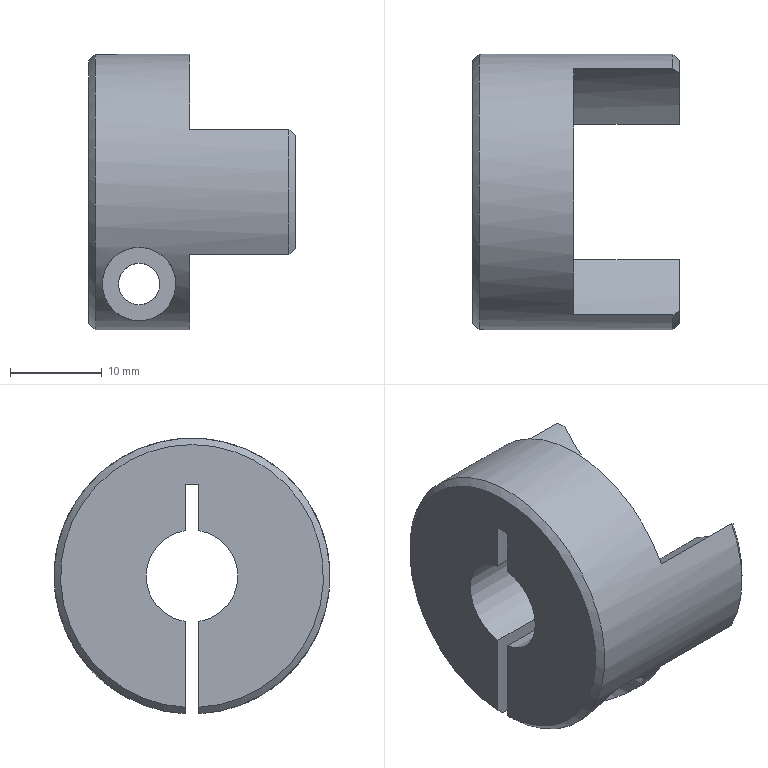Part | NX | features BREP 1 | 1 solid | 28 faces | box 22.5 x 30 x 29.981 mm | volume 7460 mm3 | cylinder 15 | plane 10 | cone 3 | commonest cylinder face diameters 4.5 x4 32.5 x4 8 x2 10 x2 15 x2 30 x1
STEP:
#1=CARTESIAN_POINT('',(5.5,0.75,-12.25));
#2=VERTEX_POINT('',#1);
#3=CARTESIAN_POINT('',(5.5,0.75,-7.75));
#4=VERTEX_POINT('',#3);
#5=CARTESIAN_POINT('',(5.5,0.75,-10.));
#6=DIRECTION('',(0.,1.,0.));
#7=DIRECTION('',(0.,0.,1.));
#8=AXIS2_PLACEMENT_3D('',#5,#6,#7);
#9=CIRCLE('',#8,2.25);
#10=EDGE_CURVE('',#2,#4,#9,.T.);
#11=ORIENTED_EDGE('',*,*,#10,.F.);
#12=CARTESIAN_POINT('',(5.5,8.657,-12.25));
#13=VERTEX_POINT('',#12);
#14=CARTESIAN_POINT('',(5.5,13.748,-12.25));
#15=DIRECTION('',(0.,1.,0.));
#16=VECTOR('',#15,1000.);
#17=LINE('',#14,#16);
#18=EDGE_CURVE('',#2,#13,#17,.T.);
#19=ORIENTED_EDGE('',*,*,#18,.T.);
#20=CARTESIAN_POINT('',(5.5,12.843,-7.75));
#21=VERTEX_POINT('',#20);
#22=CARTESIAN_POINT('',(5.5,8.657,-12.25));
#23=CARTESIAN_POINT('',(4.786,8.657,-12.25));
#24=CARTESIAN_POINT('',(3.672,9.571,-11.603));
#25=CARTESIAN_POINT('',(3.097,11.052,-10.221));
#26=CARTESIAN_POINT('',(3.478,12.411,-8.494));
#27=CARTESIAN_POINT('',(4.788,12.843,-7.75));
#28=CARTESIAN_POINT('',(5.5,12.843,-7.75));
#29=B_SPLINE_CURVE_WITH_KNOTS('',3,(#22,#23,#24,#25,#26,#27,#28),.UNSPECIFIED.,.F.,.F.,(4,1,1,1,4),(0.,0.002109,0.004218,0.006326,0.008435),.UNSPECIFIED.);
#30=EDGE_CURVE('',#13,#21,#29,.T.);
#31=ORIENTED_EDGE('',*,*,#30,.T.);
#32=CARTESIAN_POINT('',(5.5,13.748,-7.75));
#33=DIRECTION('',(0.,1.,0.));
#34=VECTOR('',#33,1000.);
#35=LINE('',#32,#34);
#36=EDGE_CURVE('',#4,#21,#35,.T.);
#37=ORIENTED_EDGE('',*,*,#36,.F.);
#38=EDGE_LOOP('',(#11,#19,#31,#37));
#39=FACE_BOUND('',#38,.T.);
#40=CARTESIAN_POINT('',(5.5,13.748,-10.));
#41=DIRECTION('',(0.,1.,0.));
#42=DIRECTION('',(0.,0.,-1.));
#43=AXIS2_PLACEMENT_3D('',#40,#41,#42);
#44=CYLINDRICAL_SURFACE('',#43,2.25);
#45=ADVANCED_FACE('',(#39),#44,.F.);
#46=CARTESIAN_POINT('',(5.5,-13.748,-6.));
#47=VERTEX_POINT('',#46);
#48=CARTESIAN_POINT('',(5.5,-5.385,-14.));
#49=VERTEX_POINT('',#48);
#50=CARTESIAN_POINT('',(5.5,-13.748,-6.));
#51=CARTESIAN_POINT('',(4.181,-13.748,-6.));
#52=CARTESIAN_POINT('',(2.328,-13.314,-7.082));
#53=CARTESIAN_POINT('',(1.48,-11.906,-9.196));
#54=CARTESIAN_POINT('',(1.476,-10.6,-10.673));
#55=CARTESIAN_POINT('',(1.92,-9.153,-11.932));
#56=CARTESIAN_POINT('',(2.686,-7.669,-12.929));
#57=CARTESIAN_POINT('',(3.738,-6.207,-13.686));
#58=CARTESIAN_POINT('',(4.838,-5.385,-14.));
#59=CARTESIAN_POINT('',(5.5,-5.385,-14.));
#60=B_SPLINE_CURVE_WITH_KNOTS('',3,(#50,#51,#52,#53,#54,#55,#56,#57,#58,#59),.UNSPECIFIED.,.F.,.F.,(4,1,1,1,1,1,1,4),(0.,0.003899,0.005849,0.007799,0.009748,0.0117,0.01365,0.0156),.UNSPECIFIED.);
#61=EDGE_CURVE('',#47,#49,#60,.T.);
#62=ORIENTED_EDGE('',*,*,#61,.T.);
#63=CARTESIAN_POINT('',(5.5,-4.75,-14.));
#64=VERTEX_POINT('',#63);
#65=CARTESIAN_POINT('',(5.5,13.748,-14.));
#66=DIRECTION('',(0.,1.,0.));
#67=VECTOR('',#66,1000.);
#68=LINE('',#65,#67);
#69=EDGE_CURVE('',#64,#49,#68,.F.);
#70=ORIENTED_EDGE('',*,*,#69,.F.);
#71=CARTESIAN_POINT('',(5.5,-4.75,-6.));
#72=VERTEX_POINT('',#71);
#73=CARTESIAN_POINT('',(5.5,-4.75,-10.));
#74=DIRECTION('',(0.,1.,0.));
#75=DIRECTION('',(0.,0.,1.));
#76=AXIS2_PLACEMENT_3D('',#73,#74,#75);
#77=CIRCLE('',#76,4.);
#78=EDGE_CURVE('',#64,#72,#77,.T.);
#79=ORIENTED_EDGE('',*,*,#78,.T.);
#80=CARTESIAN_POINT('',(5.5,13.748,-6.));
#81=DIRECTION('',(0.,1.,0.));
#82=VECTOR('',#81,1000.);
#83=LINE('',#80,#82);
#84=EDGE_CURVE('',#72,#47,#83,.F.);
#85=ORIENTED_EDGE('',*,*,#84,.T.);
#86=EDGE_LOOP('',(#62,#70,#79,#85));
#87=FACE_BOUND('',#86,.T.);
#88=CARTESIAN_POINT('',(5.5,13.748,-10.));
#89=DIRECTION('',(0.,1.,0.));
#90=DIRECTION('',(0.,0.,-1.));
#91=AXIS2_PLACEMENT_3D('',#88,#89,#90);
#92=CYLINDRICAL_SURFACE('',#91,4.);
#93=ADVANCED_FACE('',(#87),#92,.F.);
#94=CARTESIAN_POINT('',(5.5,-4.75,-12.25));
#95=VERTEX_POINT('',#94);
#96=CARTESIAN_POINT('',(5.5,-4.75,-7.75));
#97=VERTEX_POINT('',#96);
#98=CARTESIAN_POINT('',(5.5,-4.75,-10.));
#99=DIRECTION('',(0.,1.,0.));
#100=DIRECTION('',(0.,0.,1.));
#101=AXIS2_PLACEMENT_3D('',#98,#99,#100);
#102=CIRCLE('',#101,2.25);
#103=EDGE_CURVE('',#95,#97,#102,.T.);
#104=ORIENTED_EDGE('',*,*,#103,.F.);
#105=CARTESIAN_POINT('',(5.5,-0.75,-12.25));
#106=VERTEX_POINT('',#105);
#107=CARTESIAN_POINT('',(5.5,13.748,-12.25));
#108=DIRECTION('',(0.,1.,0.));
#109=VECTOR('',#108,1000.);
#110=LINE('',#107,#109);
#111=EDGE_CURVE('',#95,#106,#110,.T.);
#112=ORIENTED_EDGE('',*,*,#111,.T.);
#113=CARTESIAN_POINT('',(5.5,-0.75,-7.75));
#114=VERTEX_POINT('',#113);
#115=CARTESIAN_POINT('',(5.5,-0.75,-10.));
#116=DIRECTION('',(0.,-1.,0.));
#117=DIRECTION('',(0.,0.,-1.));
#118=AXIS2_PLACEMENT_3D('',#115,#116,#117);
#119=CIRCLE('',#118,2.25);
#120=EDGE_CURVE('',#114,#106,#119,.T.);
#121=ORIENTED_EDGE('',*,*,#120,.F.);
#122=CARTESIAN_POINT('',(5.5,13.748,-7.75));
#123=DIRECTION('',(0.,1.,0.));
#124=VECTOR('',#123,1000.);
#125=LINE('',#122,#124);
#126=EDGE_CURVE('',#97,#114,#125,.T.);
#127=ORIENTED_EDGE('',*,*,#126,.F.);
#128=EDGE_LOOP('',(#104,#112,#121,#127));
#129=FACE_BOUND('',#128,.T.);
#130=CARTESIAN_POINT('',(5.5,13.748,-10.));
#131=DIRECTION('',(0.,1.,0.));
#132=DIRECTION('',(0.,0.,-1.));
#133=AXIS2_PLACEMENT_3D('',#130,#131,#132);
#134=CYLINDRICAL_SURFACE('',#133,2.25);
#135=ADVANCED_FACE('',(#129),#134,.F.);
#136=ORIENTED_EDGE('',*,*,#120,.T.);
#137=CARTESIAN_POINT('',(5.5,-0.75,-10.));
#138=DIRECTION('',(0.,-1.,0.));
#139=DIRECTION('',(0.,0.,-1.));
#140=AXIS2_PLACEMENT_3D('',#137,#138,#139);
#141=CIRCLE('',#140,2.25);
#142=EDGE_CURVE('',#106,#114,#141,.T.);
#143=ORIENTED_EDGE('',*,*,#142,.T.);
#144=EDGE_LOOP('',(#136,#143));
#145=FACE_BOUND('',#144,.T.);
#146=CARTESIAN_POINT('',(0.7071,-0.75,-14.981));
#147=VERTEX_POINT('',#146);
#148=CARTESIAN_POINT('',(11.,-0.75,-14.981));
#149=VERTEX_POINT('',#148);
#150=CARTESIAN_POINT('',(0.,-0.75,-14.981));
#151=DIRECTION('',(1.,0.,0.));
#152=VECTOR('',#151,1000.);
#153=LINE('',#150,#152);
#154=EDGE_CURVE('',#147,#149,#153,.T.);
#155=ORIENTED_EDGE('',*,*,#154,.F.);
#156=CARTESIAN_POINT('',(0.,-0.75,-14.273));
#157=VERTEX_POINT('',#156);
#158=CARTESIAN_POINT('',(0.7071,-0.75,-14.981));
#159=CARTESIAN_POINT('',(0.4714,-0.75,-14.745));
#160=CARTESIAN_POINT('',(0.2357,-0.75,-14.509));
#161=CARTESIAN_POINT('',(0.,-0.75,-14.273));
#162=B_SPLINE_CURVE_WITH_KNOTS('',3,(#158,#159,#160,#161),.UNSPECIFIED.,.F.,.F.,(4,4),(0.,1.),.PIECEWISE_BEZIER_KNOTS.);
#163=EDGE_CURVE('',#147,#157,#162,.T.);
#164=ORIENTED_EDGE('',*,*,#163,.T.);
#165=CARTESIAN_POINT('',(0.,-0.75,-4.943));
#166=VERTEX_POINT('',#165);
#167=CARTESIAN_POINT('',(0.,-0.75,10.));
#168=DIRECTION('',(0.,0.,-1.));
#169=VECTOR('',#168,1000.);
#170=LINE('',#167,#169);
#171=EDGE_CURVE('',#166,#157,#170,.T.);
#172=ORIENTED_EDGE('',*,*,#171,.F.);
#173=CARTESIAN_POINT('',(11.,-0.75,-4.943));
#174=VERTEX_POINT('',#173);
#175=CARTESIAN_POINT('',(0.,-0.75,-4.943));
#176=DIRECTION('',(1.,0.,0.));
#177=VECTOR('',#176,1000.);
#178=LINE('',#175,#177);
#179=EDGE_CURVE('',#166,#174,#178,.T.);
#180=ORIENTED_EDGE('',*,*,#179,.T.);
#181=CARTESIAN_POINT('',(11.,-0.75,10.));
#182=DIRECTION('',(0.,0.,-1.));
#183=VECTOR('',#182,1000.);
#184=LINE('',#181,#183);
#185=EDGE_CURVE('',#174,#149,#184,.T.);
#186=ORIENTED_EDGE('',*,*,#185,.T.);
#187=EDGE_LOOP('',(#155,#164,#172,#180,#186));
#188=FACE_BOUND('',#187,.T.);
#189=CARTESIAN_POINT('',(0.,-0.75,10.));
#190=DIRECTION('',(0.,-1.,0.));
#191=DIRECTION('',(0.,0.,1.));
#192=AXIS2_PLACEMENT_3D('',#189,#190,#191);
#193=PLANE('',#192);
#194=ADVANCED_FACE('',(#145,#188),#193,.F.);
#195=CARTESIAN_POINT('',(0.,0.75,4.943));
#196=VERTEX_POINT('',#195);
#197=CARTESIAN_POINT('',(0.,0.75,10.));
#198=VERTEX_POINT('',#197);
#199=CARTESIAN_POINT('',(0.,0.75,-14.981));
#200=DIRECTION('',(0.,0.,1.));
#201=VECTOR('',#200,1000.);
#202=LINE('',#199,#201);
#203=EDGE_CURVE('',#196,#198,#202,.T.);
#204=ORIENTED_EDGE('',*,*,#203,.F.);
#205=CARTESIAN_POINT('',(11.,0.75,4.943));
#206=VERTEX_POINT('',#205);
#207=CARTESIAN_POINT('',(0.,0.75,4.943));
#208=DIRECTION('',(1.,0.,0.));
#209=VECTOR('',#208,1000.);
#210=LINE('',#207,#209);
#211=EDGE_CURVE('',#196,#206,#210,.T.);
#212=ORIENTED_EDGE('',*,*,#211,.T.);
#213=CARTESIAN_POINT('',(11.,0.75,10.));
#214=VERTEX_POINT('',#213);
#215=CARTESIAN_POINT('',(11.,0.75,-14.981));
#216=DIRECTION('',(0.,0.,1.));
#217=VECTOR('',#216,1000.);
#218=LINE('',#215,#217);
#219=EDGE_CURVE('',#206,#214,#218,.T.);
#220=ORIENTED_EDGE('',*,*,#219,.T.);
#221=CARTESIAN_POINT('',(0.,0.75,10.));
#222=DIRECTION('',(1.,0.,0.));
#223=VECTOR('',#222,1000.);
#224=LINE('',#221,#223);
#225=EDGE_CURVE('',#198,#214,#224,.T.);
#226=ORIENTED_EDGE('',*,*,#225,.F.);
#227=EDGE_LOOP('',(#204,#212,#220,#226));
#228=FACE_BOUND('',#227,.T.);
#229=CARTESIAN_POINT('',(0.,0.75,-14.981));
#230=DIRECTION('',(0.,1.,0.));
#231=DIRECTION('',(0.,0.,-1.));
#232=AXIS2_PLACEMENT_3D('',#229,#230,#231);
#233=PLANE('',#232);
#234=ADVANCED_FACE('',(#228),#233,.F.);
#235=CARTESIAN_POINT('',(11.,-0.75,4.943));
#236=VERTEX_POINT('',#235);
#237=CARTESIAN_POINT('',(11.,0.,0.));
#238=DIRECTION('',(1.,0.,0.));
#239=DIRECTION('',(0.,0.,-1.));
#240=AXIS2_PLACEMENT_3D('',#237,#238,#239);
#241=CIRCLE('',#240,5.);
#242=EDGE_CURVE('',#236,#174,#241,.T.);
#243=ORIENTED_EDGE('',*,*,#242,.F.);
#244=CARTESIAN_POINT('',(11.,-0.75,10.));
#245=VERTEX_POINT('',#244);
#246=CARTESIAN_POINT('',(11.,-0.75,10.));
#247=DIRECTION('',(0.,0.,-1.));
#248=VECTOR('',#247,1000.);
#249=LINE('',#246,#248);
#250=EDGE_CURVE('',#245,#236,#249,.T.);
#251=ORIENTED_EDGE('',*,*,#250,.F.);
#252=CARTESIAN_POINT('',(11.,0.75,10.));
#253=DIRECTION('',(0.,-1.,0.));
#254=VECTOR('',#253,1000.);
#255=LINE('',#252,#254);
#256=EDGE_CURVE('',#214,#245,#255,.T.);
#257=ORIENTED_EDGE('',*,*,#256,.F.);
#258=ORIENTED_EDGE('',*,*,#219,.F.);
#259=CARTESIAN_POINT('',(11.,0.75,-4.943));
#260=VERTEX_POINT('',#259);
#261=CARTESIAN_POINT('',(11.,0.,0.));
#262=DIRECTION('',(1.,0.,0.));
#263=DIRECTION('',(0.,0.,-1.));
#264=AXIS2_PLACEMENT_3D('',#261,#262,#263);
#265=CIRCLE('',#264,5.);
#266=EDGE_CURVE('',#260,#206,#265,.T.);
#267=ORIENTED_EDGE('',*,*,#266,.F.);
#268=CARTESIAN_POINT('',(11.,0.75,-14.981));
#269=VERTEX_POINT('',#268);
#270=CARTESIAN_POINT('',(11.,0.75,-14.981));
#271=DIRECTION('',(0.,0.,1.));
#272=VECTOR('',#271,1000.);
#273=LINE('',#270,#272);
#274=EDGE_CURVE('',#269,#260,#273,.T.);
#275=ORIENTED_EDGE('',*,*,#274,.F.);
#276=CARTESIAN_POINT('',(11.,13.381,-6.779));
#277=VERTEX_POINT('',#276);
#278=CARTESIAN_POINT('',(11.,0.,0.));
#279=DIRECTION('',(1.,0.,0.));
#280=DIRECTION('',(0.,0.,-1.));
#281=AXIS2_PLACEMENT_3D('',#278,#279,#280);
#282=CIRCLE('',#281,15.);
#283=EDGE_CURVE('',#269,#277,#282,.T.);
#284=ORIENTED_EDGE('',*,*,#283,.T.);
#285=CARTESIAN_POINT('',(11.,7.347,-1.506));
#286=VERTEX_POINT('',#285);
#287=CARTESIAN_POINT('',(11.,0.,-16.));
#288=DIRECTION('',(-1.,0.,0.));
#289=DIRECTION('',(0.,0.,-1.));
#290=AXIS2_PLACEMENT_3D('',#287,#288,#289);
#291=CIRCLE('',#290,16.25);
#292=EDGE_CURVE('',#286,#277,#291,.T.);
#293=ORIENTED_EDGE('',*,*,#292,.F.);
#294=CARTESIAN_POINT('',(11.,7.347,1.506));
#295=VERTEX_POINT('',#294);
#296=CARTESIAN_POINT('',(11.,0.,0.));
#297=DIRECTION('',(-1.,0.,0.));
#298=DIRECTION('',(0.,0.,-1.));
#299=AXIS2_PLACEMENT_3D('',#296,#297,#298);
#300=CIRCLE('',#299,7.5);
#301=EDGE_CURVE('',#295,#286,#300,.T.);
#302=ORIENTED_EDGE('',*,*,#301,.F.);
#303=CARTESIAN_POINT('',(11.,13.381,6.779));
#304=VERTEX_POINT('',#303);
#305=CARTESIAN_POINT('',(11.,0.,16.));
#306=DIRECTION('',(-1.,0.,0.));
#307=DIRECTION('',(0.,0.,-1.));
#308=AXIS2_PLACEMENT_3D('',#305,#306,#307);
#309=CIRCLE('',#308,16.25);
#310=EDGE_CURVE('',#304,#295,#309,.T.);
#311=ORIENTED_EDGE('',*,*,#310,.F.);
#312=CARTESIAN_POINT('',(11.,-13.381,6.779));
#313=VERTEX_POINT('',#312);
#314=CARTESIAN_POINT('',(11.,0.,0.));
#315=DIRECTION('',(1.,0.,0.));
#316=DIRECTION('',(0.,0.,-1.));
#317=AXIS2_PLACEMENT_3D('',#314,#315,#316);
#318=CIRCLE('',#317,15.);
#319=EDGE_CURVE('',#304,#313,#318,.T.);
#320=ORIENTED_EDGE('',*,*,#319,.T.);
#321=CARTESIAN_POINT('',(11.,-7.347,1.506));
#322=VERTEX_POINT('',#321);
#323=CARTESIAN_POINT('',(11.,0.,16.));
#324=DIRECTION('',(1.,0.,0.));
#325=DIRECTION('',(0.,0.,-1.));
#326=AXIS2_PLACEMENT_3D('',#323,#324,#325);
#327=CIRCLE('',#326,16.25);
#328=EDGE_CURVE('',#313,#322,#327,.T.);
#329=ORIENTED_EDGE('',*,*,#328,.T.);
#330=CARTESIAN_POINT('',(11.,-7.347,-1.506));
#331=VERTEX_POINT('',#330);
#332=CARTESIAN_POINT('',(11.,0.,0.));
#333=DIRECTION('',(1.,0.,0.));
#334=DIRECTION('',(0.,0.,-1.));
#335=AXIS2_PLACEMENT_3D('',#332,#333,#334);
#336=CIRCLE('',#335,7.5);
#337=EDGE_CURVE('',#322,#331,#336,.T.);
#338=ORIENTED_EDGE('',*,*,#337,.T.);
#339=CARTESIAN_POINT('',(11.,-13.381,-6.779));
#340=VERTEX_POINT('',#339);
#341=CARTESIAN_POINT('',(11.,0.,-16.));
#342=DIRECTION('',(1.,0.,0.));
#343=DIRECTION('',(0.,0.,-1.));
#344=AXIS2_PLACEMENT_3D('',#341,#342,#343);
#345=CIRCLE('',#344,16.25);
#346=EDGE_CURVE('',#331,#340,#345,.T.);
#347=ORIENTED_EDGE('',*,*,#346,.T.);
#348=CARTESIAN_POINT('',(11.,0.,0.));
#349=DIRECTION('',(1.,0.,0.));
#350=DIRECTION('',(0.,0.,-1.));
#351=AXIS2_PLACEMENT_3D('',#348,#349,#350);
#352=CIRCLE('',#351,15.);
#353=EDGE_CURVE('',#340,#149,#352,.T.);
#354=ORIENTED_EDGE('',*,*,#353,.T.);
#355=ORIENTED_EDGE('',*,*,#185,.F.);
#356=EDGE_LOOP('',(#243,#251,#257,#258,#267,#275,#284,#293,#302,#311,#320,#329,#338,#347,#354,#355));
#357=FACE_BOUND('',#356,.T.);
#358=CARTESIAN_POINT('',(11.,0.,8.));
#359=DIRECTION('',(1.,0.,0.));
#360=DIRECTION('',(0.,0.,1.));
#361=AXIS2_PLACEMENT_3D('',#358,#359,#360);
#362=PLANE('',#361);
#363=ADVANCED_FACE('',(#357),#362,.T.);
#364=CARTESIAN_POINT('',(5.5,12.843,-7.75));
#365=CARTESIAN_POINT('',(6.211,12.843,-7.75));
#366=CARTESIAN_POINT('',(7.521,12.413,-8.492));
#367=CARTESIAN_POINT('',(7.904,11.052,-10.221));
#368=CARTESIAN_POINT('',(7.328,9.571,-11.603));
#369=CARTESIAN_POINT('',(6.214,8.657,-12.25));
#370=CARTESIAN_POINT('',(5.5,8.657,-12.25));
#371=B_SPLINE_CURVE_WITH_KNOTS('',3,(#364,#365,#366,#367,#368,#369,#370),.UNSPECIFIED.,.F.,.F.,(4,1,1,1,4),(0.,0.0021,0.004201,0.006301,0.008402),.UNSPECIFIED.);
#372=EDGE_CURVE('',#21,#13,#371,.T.);
#373=ORIENTED_EDGE('',*,*,#372,.F.);
#374=ORIENTED_EDGE('',*,*,#30,.F.);
#375=EDGE_LOOP('',(#373,#374));
#376=FACE_BOUND('',#375,.T.);
#377=ORIENTED_EDGE('',*,*,#61,.F.);
#378=CARTESIAN_POINT('',(5.5,-5.385,-14.));
#379=CARTESIAN_POINT('',(6.165,-5.385,-14.));
#380=CARTESIAN_POINT('',(7.265,-6.212,-13.683));
#381=CARTESIAN_POINT('',(8.31,-7.662,-12.934));
#382=CARTESIAN_POINT('',(9.083,-9.162,-11.923));
#383=CARTESIAN_POINT('',(9.667,-11.064,-10.283));
#384=CARTESIAN_POINT('',(9.299,-13.162,-7.484));
#385=CARTESIAN_POINT('',(6.823,-13.748,-6.));
#386=CARTESIAN_POINT('',(5.5,-13.748,-6.));
#387=B_SPLINE_CURVE_WITH_KNOTS('',3,(#378,#379,#380,#381,#382,#383,#384,#385,#386),.UNSPECIFIED.,.F.,.F.,(4,1,1,1,1,1,4),(0.,0.001957,0.003915,0.005872,0.00783,0.01174,0.01566),.UNSPECIFIED.);
#388=EDGE_CURVE('',#49,#47,#387,.T.);
#389=ORIENTED_EDGE('',*,*,#388,.F.);
#390=EDGE_LOOP('',(#377,#389));
#391=FACE_BOUND('',#390,.T.);
#392=CARTESIAN_POINT('',(21.793,-13.381,-6.779));
#393=VERTEX_POINT('',#392);
#394=CARTESIAN_POINT('',(11.,-13.381,-6.779));
#395=DIRECTION('',(1.,0.,0.));
#396=VECTOR('',#395,1000.);
#397=LINE('',#394,#396);
#398=EDGE_CURVE('',#340,#393,#397,.T.);
#399=ORIENTED_EDGE('',*,*,#398,.T.);
#400=CARTESIAN_POINT('',(21.793,-13.381,6.779));
#401=VERTEX_POINT('',#400);
#402=CARTESIAN_POINT('',(21.793,0.,0.));
#403=DIRECTION('',(-1.,0.,0.));
#404=DIRECTION('',(0.,0.,-1.));
#405=AXIS2_PLACEMENT_3D('',#402,#403,#404);
#406=CIRCLE('',#405,15.);
#407=EDGE_CURVE('',#393,#401,#406,.T.);
#408=ORIENTED_EDGE('',*,*,#407,.T.);
#409=CARTESIAN_POINT('',(11.,-13.381,6.779));
#410=DIRECTION('',(1.,0.,0.));
#411=VECTOR('',#410,1000.);
#412=LINE('',#409,#411);
#413=EDGE_CURVE('',#313,#401,#412,.T.);
#414=ORIENTED_EDGE('',*,*,#413,.F.);
#415=ORIENTED_EDGE('',*,*,#319,.F.);
#416=CARTESIAN_POINT('',(21.793,13.381,6.779));
#417=VERTEX_POINT('',#416);
#418=CARTESIAN_POINT('',(22.5,13.381,6.779));
#419=DIRECTION('',(-1.,0.,0.));
#420=VECTOR('',#419,1000.);
#421=LINE('',#418,#420);
#422=EDGE_CURVE('',#417,#304,#421,.T.);
#423=ORIENTED_EDGE('',*,*,#422,.F.);
#424=CARTESIAN_POINT('',(21.793,13.381,-6.779));
#425=VERTEX_POINT('',#424);
#426=CARTESIAN_POINT('',(21.793,0.,0.));
#427=DIRECTION('',(-1.,0.,0.));
#428=DIRECTION('',(0.,0.,-1.));
#429=AXIS2_PLACEMENT_3D('',#426,#427,#428);
#430=CIRCLE('',#429,15.);
#431=EDGE_CURVE('',#417,#425,#430,.T.);
#432=ORIENTED_EDGE('',*,*,#431,.T.);
#433=CARTESIAN_POINT('',(22.5,13.381,-6.779));
#434=DIRECTION('',(-1.,0.,0.));
#435=VECTOR('',#434,1000.);
#436=LINE('',#433,#435);
#437=EDGE_CURVE('',#425,#277,#436,.T.);
#438=ORIENTED_EDGE('',*,*,#437,.T.);
#439=ORIENTED_EDGE('',*,*,#283,.F.);
#440=CARTESIAN_POINT('',(0.7071,0.75,-14.981));
#441=VERTEX_POINT('',#440);
#442=CARTESIAN_POINT('',(0.,0.75,-14.981));
#443=DIRECTION('',(1.,0.,0.));
#444=VECTOR('',#443,1000.);
#445=LINE('',#442,#444);
#446=EDGE_CURVE('',#441,#269,#445,.T.);
#447=ORIENTED_EDGE('',*,*,#446,.F.);
#448=CARTESIAN_POINT('',(0.7071,0.,0.));
#449=DIRECTION('',(1.,0.,0.));
#450=DIRECTION('',(0.,0.,1.));
#451=AXIS2_PLACEMENT_3D('',#448,#449,#450);
#452=CIRCLE('',#451,15.);
#453=EDGE_CURVE('',#441,#147,#452,.T.);
#454=ORIENTED_EDGE('',*,*,#453,.T.);
#455=ORIENTED_EDGE('',*,*,#154,.T.);
#456=ORIENTED_EDGE('',*,*,#353,.F.);
#457=EDGE_LOOP('',(#399,#408,#414,#415,#423,#432,#438,#439,#447,#454,#455,#456));
#458=FACE_BOUND('',#457,.T.);
#459=CARTESIAN_POINT('',(0.,0.,0.));
#460=DIRECTION('',(1.,0.,0.));
#461=DIRECTION('',(0.,0.,1.));
#462=AXIS2_PLACEMENT_3D('',#459,#460,#461);
#463=CYLINDRICAL_SURFACE('',#462,15.);
#464=ADVANCED_FACE('',(#376,#391,#458),#463,.T.);
#465=ORIENTED_EDGE('',*,*,#171,.T.);
#466=CARTESIAN_POINT('',(0.,0.75,-14.273));
#467=VERTEX_POINT('',#466);
#468=CARTESIAN_POINT('',(0.,0.,0.));
#469=DIRECTION('',(-1.,0.,0.));
#470=DIRECTION('',(0.,0.,1.));
#471=AXIS2_PLACEMENT_3D('',#468,#469,#470);
#472=CIRCLE('',#471,14.293);
#473=EDGE_CURVE('',#157,#467,#472,.T.);
#474=ORIENTED_EDGE('',*,*,#473,.T.);
#475=CARTESIAN_POINT('',(0.,0.75,-4.943));
#476=VERTEX_POINT('',#475);
#477=CARTESIAN_POINT('',(0.,0.75,-14.981));
#478=DIRECTION('',(0.,0.,1.));
#479=VECTOR('',#478,1000.);
#480=LINE('',#477,#479);
#481=EDGE_CURVE('',#467,#476,#480,.T.);
#482=ORIENTED_EDGE('',*,*,#481,.T.);
#483=CARTESIAN_POINT('',(0.,0.,0.));
#484=DIRECTION('',(1.,0.,0.));
#485=DIRECTION('',(0.,0.,-1.));
#486=AXIS2_PLACEMENT_3D('',#483,#484,#485);
#487=CIRCLE('',#486,5.);
#488=EDGE_CURVE('',#476,#196,#487,.T.);
#489=ORIENTED_EDGE('',*,*,#488,.T.);
#490=ORIENTED_EDGE('',*,*,#203,.T.);
#491=CARTESIAN_POINT('',(0.,-0.75,10.));
#492=VERTEX_POINT('',#491);
#493=CARTESIAN_POINT('',(0.,0.75,10.));
#494=DIRECTION('',(0.,-1.,0.));
#495=VECTOR('',#494,1000.);
#496=LINE('',#493,#495);
#497=EDGE_CURVE('',#198,#492,#496,.T.);
#498=ORIENTED_EDGE('',*,*,#497,.T.);
#499=CARTESIAN_POINT('',(0.,-0.75,4.943));
#500=VERTEX_POINT('',#499);
#501=CARTESIAN_POINT('',(0.,-0.75,10.));
#502=DIRECTION('',(0.,0.,-1.));
#503=VECTOR('',#502,1000.);
#504=LINE('',#501,#503);
#505=EDGE_CURVE('',#492,#500,#504,.T.);
#506=ORIENTED_EDGE('',*,*,#505,.T.);
#507=CARTESIAN_POINT('',(0.,0.,0.));
#508=DIRECTION('',(1.,0.,0.));
#509=DIRECTION('',(0.,0.,-1.));
#510=AXIS2_PLACEMENT_3D('',#507,#508,#509);
#511=CIRCLE('',#510,5.);
#512=EDGE_CURVE('',#500,#166,#511,.T.);
#513=ORIENTED_EDGE('',*,*,#512,.T.);
#514=EDGE_LOOP('',(#465,#474,#482,#489,#490,#498,#506,#513));
#515=FACE_BOUND('',#514,.T.);
#516=CARTESIAN_POINT('',(0.,15.,0.));
#517=DIRECTION('',(-1.,0.,0.));
#518=DIRECTION('',(0.,0.,-1.));
#519=AXIS2_PLACEMENT_3D('',#516,#517,#518);
#520=PLANE('',#519);
#521=ADVANCED_FACE('',(#515),#520,.T.);
#522=CARTESIAN_POINT('',(22.5,-12.911,6.132));
#523=VERTEX_POINT('',#522);
#524=CARTESIAN_POINT('',(22.5,-7.347,1.506));
#525=VERTEX_POINT('',#524);
#526=CARTESIAN_POINT('',(22.5,0.,16.));
#527=DIRECTION('',(1.,0.,0.));
#528=DIRECTION('',(0.,0.,-1.));
#529=AXIS2_PLACEMENT_3D('',#526,#527,#528);
#530=CIRCLE('',#529,16.25);
#531=EDGE_CURVE('',#523,#525,#530,.T.);
#532=ORIENTED_EDGE('',*,*,#531,.F.);
#533=CARTESIAN_POINT('',(22.5,-12.911,-6.132));
#534=VERTEX_POINT('',#533);
#535=CARTESIAN_POINT('',(22.5,0.,0.));
#536=DIRECTION('',(1.,0.,0.));
#537=DIRECTION('',(0.,0.,-1.));
#538=AXIS2_PLACEMENT_3D('',#535,#536,#537);
#539=CIRCLE('',#538,14.293);
#540=EDGE_CURVE('',#523,#534,#539,.T.);
#541=ORIENTED_EDGE('',*,*,#540,.T.);
#542=CARTESIAN_POINT('',(22.5,-7.347,-1.506));
#543=VERTEX_POINT('',#542);
#544=CARTESIAN_POINT('',(22.5,0.,-16.));
#545=DIRECTION('',(1.,0.,0.));
#546=DIRECTION('',(0.,0.,-1.));
#547=AXIS2_PLACEMENT_3D('',#544,#545,#546);
#548=CIRCLE('',#547,16.25);
#549=EDGE_CURVE('',#543,#534,#548,.T.);
#550=ORIENTED_EDGE('',*,*,#549,.F.);
#551=CARTESIAN_POINT('',(22.5,0.,0.));
#552=DIRECTION('',(1.,0.,0.));
#553=DIRECTION('',(0.,0.,-1.));
#554=AXIS2_PLACEMENT_3D('',#551,#552,#553);
#555=CIRCLE('',#554,7.5);
#556=EDGE_CURVE('',#525,#543,#555,.T.);
#557=ORIENTED_EDGE('',*,*,#556,.F.);
#558=EDGE_LOOP('',(#532,#541,#550,#557));
#559=FACE_BOUND('',#558,.T.);
#560=CARTESIAN_POINT('',(22.5,0.,0.));
#561=DIRECTION('',(1.,0.,0.));
#562=DIRECTION('',(0.,0.,1.));
#563=AXIS2_PLACEMENT_3D('',#560,#561,#562);
#564=PLANE('',#563);
#565=ADVANCED_FACE('',(#559),#564,.T.);
#566=ORIENTED_EDGE('',*,*,#549,.T.);
#567=CARTESIAN_POINT('',(22.5,-12.911,-6.132));
#568=CARTESIAN_POINT('',(22.263,-13.072,-6.343));
#569=CARTESIAN_POINT('',(22.028,-13.229,-6.559));
#570=CARTESIAN_POINT('',(21.793,-13.381,-6.779));
#571=B_SPLINE_CURVE_WITH_KNOTS('',3,(#567,#568,#569,#570),.UNSPECIFIED.,.F.,.F.,(4,4),(0.,1.),.PIECEWISE_BEZIER_KNOTS.);
#572=EDGE_CURVE('',#534,#393,#571,.T.);
#573=ORIENTED_EDGE('',*,*,#572,.T.);
#574=ORIENTED_EDGE('',*,*,#398,.F.);
#575=ORIENTED_EDGE('',*,*,#346,.F.);
#576=CARTESIAN_POINT('',(11.,-7.347,-1.506));
#577=DIRECTION('',(1.,0.,0.));
#578=VECTOR('',#577,1000.);
#579=LINE('',#576,#578);
#580=EDGE_CURVE('',#331,#543,#579,.T.);
#581=ORIENTED_EDGE('',*,*,#580,.T.);
#582=EDGE_LOOP('',(#566,#573,#574,#575,#581));
#583=FACE_BOUND('',#582,.T.);
#584=CARTESIAN_POINT('',(11.,0.,-16.));
#585=DIRECTION('',(1.,0.,0.));
#586=DIRECTION('',(0.,0.,1.));
#587=AXIS2_PLACEMENT_3D('',#584,#585,#586);
#588=CYLINDRICAL_SURFACE('',#587,16.25);
#589=ADVANCED_FACE('',(#583),#588,.F.);
#590=ORIENTED_EDGE('',*,*,#556,.T.);
#591=ORIENTED_EDGE('',*,*,#580,.F.);
#592=ORIENTED_EDGE('',*,*,#337,.F.);
#593=CARTESIAN_POINT('',(11.,-7.347,1.506));
#594=DIRECTION('',(1.,0.,0.));
#595=VECTOR('',#594,1000.);
#596=LINE('',#593,#595);
#597=EDGE_CURVE('',#322,#525,#596,.T.);
#598=ORIENTED_EDGE('',*,*,#597,.T.);
#599=EDGE_LOOP('',(#590,#591,#592,#598));
#600=FACE_BOUND('',#599,.T.);
#601=CARTESIAN_POINT('',(11.,0.,0.));
#602=DIRECTION('',(1.,0.,0.));
#603=DIRECTION('',(0.,0.,1.));
#604=AXIS2_PLACEMENT_3D('',#601,#602,#603);
#605=CYLINDRICAL_SURFACE('',#604,7.5);
#606=ADVANCED_FACE('',(#600),#605,.F.);
#607=ORIENTED_EDGE('',*,*,#413,.T.);
#608=CARTESIAN_POINT('',(21.793,-13.381,6.779));
#609=CARTESIAN_POINT('',(22.028,-13.229,6.559));
#610=CARTESIAN_POINT('',(22.263,-13.072,6.343));
#611=CARTESIAN_POINT('',(22.5,-12.911,6.132));
#612=B_SPLINE_CURVE_WITH_KNOTS('',3,(#608,#609,#610,#611),.UNSPECIFIED.,.F.,.F.,(4,4),(0.,1.),.PIECEWISE_BEZIER_KNOTS.);
#613=EDGE_CURVE('',#401,#523,#612,.T.);
#614=ORIENTED_EDGE('',*,*,#613,.T.);
#615=ORIENTED_EDGE('',*,*,#531,.T.);
#616=ORIENTED_EDGE('',*,*,#597,.F.);
#617=ORIENTED_EDGE('',*,*,#328,.F.);
#618=EDGE_LOOP('',(#607,#614,#615,#616,#617));
#619=FACE_BOUND('',#618,.T.);
#620=CARTESIAN_POINT('',(11.,0.,16.));
#621=DIRECTION('',(1.,0.,0.));
#622=DIRECTION('',(0.,0.,1.));
#623=AXIS2_PLACEMENT_3D('',#620,#621,#622);
#624=CYLINDRICAL_SURFACE('',#623,16.25);
#625=ADVANCED_FACE('',(#619),#624,.F.);
#626=ORIENTED_EDGE('',*,*,#250,.T.);
#627=CARTESIAN_POINT('',(0.,-0.75,4.943));
#628=DIRECTION('',(1.,0.,0.));
#629=VECTOR('',#628,1000.);
#630=LINE('',#627,#629);
#631=EDGE_CURVE('',#500,#236,#630,.T.);
#632=ORIENTED_EDGE('',*,*,#631,.F.);
#633=ORIENTED_EDGE('',*,*,#505,.F.);
#634=CARTESIAN_POINT('',(0.,-0.75,10.));
#635=DIRECTION('',(1.,0.,0.));
#636=VECTOR('',#635,1000.);
#637=LINE('',#634,#636);
#638=EDGE_CURVE('',#492,#245,#637,.T.);
#639=ORIENTED_EDGE('',*,*,#638,.T.);
#640=EDGE_LOOP('',(#626,#632,#633,#639));
#641=FACE_BOUND('',#640,.T.);
#642=CARTESIAN_POINT('',(0.,-0.75,10.));
#643=DIRECTION('',(0.,-1.,0.));
#644=DIRECTION('',(0.,0.,1.));
#645=AXIS2_PLACEMENT_3D('',#642,#643,#644);
#646=PLANE('',#645);
#647=ADVANCED_FACE('',(#641),#646,.F.);
#648=ORIENTED_EDGE('',*,*,#256,.T.);
#649=ORIENTED_EDGE('',*,*,#638,.F.);
#650=ORIENTED_EDGE('',*,*,#497,.F.);
#651=ORIENTED_EDGE('',*,*,#225,.T.);
#652=EDGE_LOOP('',(#648,#649,#650,#651));
#653=FACE_BOUND('',#652,.T.);
#654=CARTESIAN_POINT('',(0.,0.75,10.));
#655=DIRECTION('',(0.,0.,1.));
#656=DIRECTION('',(-1.,0.,0.));
#657=AXIS2_PLACEMENT_3D('',#654,#655,#656);
#658=PLANE('',#657);
#659=ADVANCED_FACE('',(#653),#658,.F.);
#660=CARTESIAN_POINT('',(5.5,0.75,-10.));
#661=DIRECTION('',(0.,1.,0.));
#662=DIRECTION('',(0.,0.,1.));
#663=AXIS2_PLACEMENT_3D('',#660,#661,#662);
#664=CIRCLE('',#663,2.25);
#665=EDGE_CURVE('',#4,#2,#664,.T.);
#666=ORIENTED_EDGE('',*,*,#665,.T.);
#667=ORIENTED_EDGE('',*,*,#10,.T.);
#668=EDGE_LOOP('',(#666,#667));
#669=FACE_BOUND('',#668,.T.);
#670=ORIENTED_EDGE('',*,*,#481,.F.);
#671=CARTESIAN_POINT('',(0.,0.75,-14.273));
#672=CARTESIAN_POINT('',(0.2357,0.75,-14.509));
#673=CARTESIAN_POINT('',(0.4714,0.75,-14.745));
#674=CARTESIAN_POINT('',(0.7071,0.75,-14.981));
#675=B_SPLINE_CURVE_WITH_KNOTS('',3,(#671,#672,#673,#674),.UNSPECIFIED.,.F.,.F.,(4,4),(0.,1.),.PIECEWISE_BEZIER_KNOTS.);
#676=EDGE_CURVE('',#467,#441,#675,.T.);
#677=ORIENTED_EDGE('',*,*,#676,.T.);
#678=ORIENTED_EDGE('',*,*,#446,.T.);
#679=ORIENTED_EDGE('',*,*,#274,.T.);
#680=CARTESIAN_POINT('',(0.,0.75,-4.943));
#681=DIRECTION('',(1.,0.,0.));
#682=VECTOR('',#681,1000.);
#683=LINE('',#680,#682);
#684=EDGE_CURVE('',#476,#260,#683,.T.);
#685=ORIENTED_EDGE('',*,*,#684,.F.);
#686=EDGE_LOOP('',(#670,#677,#678,#679,#685));
#687=FACE_BOUND('',#686,.T.);
#688=CARTESIAN_POINT('',(0.,0.75,-14.981));
#689=DIRECTION('',(0.,1.,0.));
#690=DIRECTION('',(0.,0.,-1.));
#691=AXIS2_PLACEMENT_3D('',#688,#689,#690);
#692=PLANE('',#691);
#693=ADVANCED_FACE('',(#669,#687),#692,.F.);
#694=ORIENTED_EDGE('',*,*,#437,.F.);
#695=CARTESIAN_POINT('',(22.5,12.911,-6.132));
#696=VERTEX_POINT('',#695);
#697=CARTESIAN_POINT('',(21.793,13.381,-6.779));
#698=CARTESIAN_POINT('',(22.028,13.229,-6.559));
#699=CARTESIAN_POINT('',(22.263,13.072,-6.343));
#700=CARTESIAN_POINT('',(22.5,12.911,-6.132));
#701=B_SPLINE_CURVE_WITH_KNOTS('',3,(#697,#698,#699,#700),.UNSPECIFIED.,.F.,.F.,(4,4),(0.,1.),.PIECEWISE_BEZIER_KNOTS.);
#702=EDGE_CURVE('',#425,#696,#701,.T.);
#703=ORIENTED_EDGE('',*,*,#702,.T.);
#704=CARTESIAN_POINT('',(22.5,7.347,-1.506));
#705=VERTEX_POINT('',#704);
#706=CARTESIAN_POINT('',(22.5,0.,-16.));
#707=DIRECTION('',(-1.,0.,0.));
#708=DIRECTION('',(0.,0.,-1.));
#709=AXIS2_PLACEMENT_3D('',#706,#707,#708);
#710=CIRCLE('',#709,16.25);
#711=EDGE_CURVE('',#705,#696,#710,.T.);
#712=ORIENTED_EDGE('',*,*,#711,.F.);
#713=CARTESIAN_POINT('',(22.5,7.347,-1.506));
#714=DIRECTION('',(-1.,0.,0.));
#715=VECTOR('',#714,1000.);
#716=LINE('',#713,#715);
#717=EDGE_CURVE('',#705,#286,#716,.T.);
#718=ORIENTED_EDGE('',*,*,#717,.T.);
#719=ORIENTED_EDGE('',*,*,#292,.T.);
#720=EDGE_LOOP('',(#694,#703,#712,#718,#719));
#721=FACE_BOUND('',#720,.T.);
#722=CARTESIAN_POINT('',(22.5,0.,-16.));
#723=DIRECTION('',(-1.,0.,0.));
#724=DIRECTION('',(0.,0.,-1.));
#725=AXIS2_PLACEMENT_3D('',#722,#723,#724);
#726=CYLINDRICAL_SURFACE('',#725,16.25);
#727=ADVANCED_FACE('',(#721),#726,.F.);
#728=CARTESIAN_POINT('',(22.5,12.911,6.132));
#729=VERTEX_POINT('',#728);
#730=CARTESIAN_POINT('',(22.5,7.347,1.506));
#731=VERTEX_POINT('',#730);
#732=CARTESIAN_POINT('',(22.5,0.,16.));
#733=DIRECTION('',(-1.,0.,0.));
#734=DIRECTION('',(0.,0.,-1.));
#735=AXIS2_PLACEMENT_3D('',#732,#733,#734);
#736=CIRCLE('',#735,16.25);
#737=EDGE_CURVE('',#729,#731,#736,.T.);
#738=ORIENTED_EDGE('',*,*,#737,.F.);
#739=CARTESIAN_POINT('',(22.5,12.911,6.132));
#740=CARTESIAN_POINT('',(22.263,13.072,6.343));
#741=CARTESIAN_POINT('',(22.028,13.229,6.559));
#742=CARTESIAN_POINT('',(21.793,13.381,6.779));
#743=B_SPLINE_CURVE_WITH_KNOTS('',3,(#739,#740,#741,#742),.UNSPECIFIED.,.F.,.F.,(4,4),(0.,1.),.PIECEWISE_BEZIER_KNOTS.);
#744=EDGE_CURVE('',#729,#417,#743,.T.);
#745=ORIENTED_EDGE('',*,*,#744,.T.);
#746=ORIENTED_EDGE('',*,*,#422,.T.);
#747=ORIENTED_EDGE('',*,*,#310,.T.);
#748=CARTESIAN_POINT('',(22.5,7.347,1.506));
#749=DIRECTION('',(-1.,0.,0.));
#750=VECTOR('',#749,1000.);
#751=LINE('',#748,#750);
#752=EDGE_CURVE('',#731,#295,#751,.T.);
#753=ORIENTED_EDGE('',*,*,#752,.F.);
#754=EDGE_LOOP('',(#738,#745,#746,#747,#753));
#755=FACE_BOUND('',#754,.T.);
#756=CARTESIAN_POINT('',(22.5,0.,16.));
#757=DIRECTION('',(-1.,0.,0.));
#758=DIRECTION('',(0.,0.,-1.));
#759=AXIS2_PLACEMENT_3D('',#756,#757,#758);
#760=CYLINDRICAL_SURFACE('',#759,16.25);
#761=ADVANCED_FACE('',(#755),#760,.F.);
#762=ORIENTED_EDGE('',*,*,#301,.T.);
#763=ORIENTED_EDGE('',*,*,#717,.F.);
#764=CARTESIAN_POINT('',(22.5,0.,0.));
#765=DIRECTION('',(-1.,0.,0.));
#766=DIRECTION('',(0.,0.,-1.));
#767=AXIS2_PLACEMENT_3D('',#764,#765,#766);
#768=CIRCLE('',#767,7.5);
#769=EDGE_CURVE('',#731,#705,#768,.T.);
#770=ORIENTED_EDGE('',*,*,#769,.F.);
#771=ORIENTED_EDGE('',*,*,#752,.T.);
#772=EDGE_LOOP('',(#762,#763,#770,#771));
#773=FACE_BOUND('',#772,.T.);
#774=CARTESIAN_POINT('',(22.5,0.,0.));
#775=DIRECTION('',(-1.,0.,0.));
#776=DIRECTION('',(0.,0.,-1.));
#777=AXIS2_PLACEMENT_3D('',#774,#775,#776);
#778=CYLINDRICAL_SURFACE('',#777,7.5);
#779=ADVANCED_FACE('',(#773),#778,.F.);
#780=ORIENTED_EDGE('',*,*,#711,.T.);
#781=CARTESIAN_POINT('',(22.5,0.,0.));
#782=DIRECTION('',(1.,0.,0.));
#783=DIRECTION('',(0.,0.,-1.));
#784=AXIS2_PLACEMENT_3D('',#781,#782,#783);
#785=CIRCLE('',#784,14.293);
#786=EDGE_CURVE('',#696,#729,#785,.T.);
#787=ORIENTED_EDGE('',*,*,#786,.T.);
#788=ORIENTED_EDGE('',*,*,#737,.T.);
#789=ORIENTED_EDGE('',*,*,#769,.T.);
#790=EDGE_LOOP('',(#780,#787,#788,#789));
#791=FACE_BOUND('',#790,.T.);
#792=CARTESIAN_POINT('',(22.5,0.,-8.));
#793=DIRECTION('',(1.,0.,0.));
#794=DIRECTION('',(0.,0.,1.));
#795=AXIS2_PLACEMENT_3D('',#792,#793,#794);
#796=PLANE('',#795);
#797=ADVANCED_FACE('',(#791),#796,.T.);
#798=ORIENTED_EDGE('',*,*,#266,.T.);
#799=ORIENTED_EDGE('',*,*,#211,.F.);
#800=ORIENTED_EDGE('',*,*,#488,.F.);
#801=ORIENTED_EDGE('',*,*,#684,.T.);
#802=EDGE_LOOP('',(#798,#799,#800,#801));
#803=FACE_BOUND('',#802,.T.);
#804=CARTESIAN_POINT('',(0.,0.,0.));
#805=DIRECTION('',(1.,0.,0.));
#806=DIRECTION('',(0.,0.,1.));
#807=AXIS2_PLACEMENT_3D('',#804,#805,#806);
#808=CYLINDRICAL_SURFACE('',#807,5.);
#809=ADVANCED_FACE('',(#803),#808,.F.);
#810=ORIENTED_EDGE('',*,*,#242,.T.);
#811=ORIENTED_EDGE('',*,*,#179,.F.);
#812=ORIENTED_EDGE('',*,*,#512,.F.);
#813=ORIENTED_EDGE('',*,*,#631,.T.);
#814=EDGE_LOOP('',(#810,#811,#812,#813));
#815=FACE_BOUND('',#814,.T.);
#816=CARTESIAN_POINT('',(0.,0.,0.));
#817=DIRECTION('',(1.,0.,0.));
#818=DIRECTION('',(0.,0.,1.));
#819=AXIS2_PLACEMENT_3D('',#816,#817,#818);
#820=CYLINDRICAL_SURFACE('',#819,5.);
#821=ADVANCED_FACE('',(#815),#820,.F.);
#822=ORIENTED_EDGE('',*,*,#111,.F.);
#823=CARTESIAN_POINT('',(5.5,-4.75,-10.));
#824=DIRECTION('',(0.,1.,0.));
#825=DIRECTION('',(0.,0.,1.));
#826=AXIS2_PLACEMENT_3D('',#823,#824,#825);
#827=CIRCLE('',#826,2.25);
#828=EDGE_CURVE('',#97,#95,#827,.T.);
#829=ORIENTED_EDGE('',*,*,#828,.F.);
#830=ORIENTED_EDGE('',*,*,#126,.T.);
#831=ORIENTED_EDGE('',*,*,#142,.F.);
#832=EDGE_LOOP('',(#822,#829,#830,#831));
#833=FACE_BOUND('',#832,.T.);
#834=CARTESIAN_POINT('',(5.5,13.748,-10.));
#835=DIRECTION('',(0.,1.,0.));
#836=DIRECTION('',(0.,0.,-1.));
#837=AXIS2_PLACEMENT_3D('',#834,#835,#836);
#838=CYLINDRICAL_SURFACE('',#837,2.25);
#839=ADVANCED_FACE('',(#833),#838,.F.);
#840=CARTESIAN_POINT('',(5.5,-4.75,-10.));
#841=DIRECTION('',(0.,1.,0.));
#842=DIRECTION('',(0.,0.,1.));
#843=AXIS2_PLACEMENT_3D('',#840,#841,#842);
#844=CIRCLE('',#843,4.);
#845=EDGE_CURVE('',#72,#64,#844,.T.);
#846=ORIENTED_EDGE('',*,*,#845,.F.);
#847=ORIENTED_EDGE('',*,*,#78,.F.);
#848=EDGE_LOOP('',(#846,#847));
#849=FACE_BOUND('',#848,.T.);
#850=ORIENTED_EDGE('',*,*,#828,.T.);
#851=ORIENTED_EDGE('',*,*,#103,.T.);
#852=EDGE_LOOP('',(#850,#851));
#853=FACE_BOUND('',#852,.T.);
#854=CARTESIAN_POINT('',(9.5,-4.75,-10.));
#855=DIRECTION('',(0.,1.,0.));
#856=DIRECTION('',(0.,0.,-1.));
#857=AXIS2_PLACEMENT_3D('',#854,#855,#856);
#858=PLANE('',#857);
#859=ADVANCED_FACE('',(#849,#853),#858,.F.);
#860=ORIENTED_EDGE('',*,*,#69,.T.);
#861=ORIENTED_EDGE('',*,*,#388,.T.);
#862=ORIENTED_EDGE('',*,*,#84,.F.);
#863=ORIENTED_EDGE('',*,*,#845,.T.);
#864=EDGE_LOOP('',(#860,#861,#862,#863));
#865=FACE_BOUND('',#864,.T.);
#866=CARTESIAN_POINT('',(5.5,13.748,-10.));
#867=DIRECTION('',(0.,1.,0.));
#868=DIRECTION('',(0.,0.,-1.));
#869=AXIS2_PLACEMENT_3D('',#866,#867,#868);
#870=CYLINDRICAL_SURFACE('',#869,4.);
#871=ADVANCED_FACE('',(#865),#870,.F.);
#872=ORIENTED_EDGE('',*,*,#18,.F.);
#873=ORIENTED_EDGE('',*,*,#665,.F.);
#874=ORIENTED_EDGE('',*,*,#36,.T.);
#875=ORIENTED_EDGE('',*,*,#372,.T.);
#876=EDGE_LOOP('',(#872,#873,#874,#875));
#877=FACE_BOUND('',#876,.T.);
#878=CARTESIAN_POINT('',(5.5,13.748,-10.));
#879=DIRECTION('',(0.,1.,0.));
#880=DIRECTION('',(0.,0.,-1.));
#881=AXIS2_PLACEMENT_3D('',#878,#879,#880);
#882=CYLINDRICAL_SURFACE('',#881,2.25);
#883=ADVANCED_FACE('',(#877),#882,.F.);
#884=ORIENTED_EDGE('',*,*,#613,.F.);
#885=ORIENTED_EDGE('',*,*,#407,.F.);
#886=ORIENTED_EDGE('',*,*,#572,.F.);
#887=ORIENTED_EDGE('',*,*,#540,.F.);
#888=EDGE_LOOP('',(#884,#885,#886,#887));
#889=FACE_BOUND('',#888,.T.);
#890=CARTESIAN_POINT('',(22.5,0.,0.));
#891=DIRECTION('',(-1.,0.,0.));
#892=DIRECTION('',(0.,0.,-1.));
#893=AXIS2_PLACEMENT_3D('',#890,#891,#892);
#894=CONICAL_SURFACE('',#893,14.293,0.7854);
#895=ADVANCED_FACE('',(#889),#894,.T.);
#896=ORIENTED_EDGE('',*,*,#676,.F.);
#897=ORIENTED_EDGE('',*,*,#473,.F.);
#898=ORIENTED_EDGE('',*,*,#163,.F.);
#899=ORIENTED_EDGE('',*,*,#453,.F.);
#900=EDGE_LOOP('',(#896,#897,#898,#899));
#901=FACE_BOUND('',#900,.T.);
#902=CARTESIAN_POINT('',(0.7071,0.,0.));
#903=DIRECTION('',(1.,0.,0.));
#904=DIRECTION('',(0.,0.,1.));
#905=AXIS2_PLACEMENT_3D('',#902,#903,#904);
#906=CONICAL_SURFACE('',#905,15.,0.7854);
#907=ADVANCED_FACE('',(#901),#906,.T.);
#908=ORIENTED_EDGE('',*,*,#702,.F.);
#909=ORIENTED_EDGE('',*,*,#431,.F.);
#910=ORIENTED_EDGE('',*,*,#744,.F.);
#911=ORIENTED_EDGE('',*,*,#786,.F.);
#912=EDGE_LOOP('',(#908,#909,#910,#911));
#913=FACE_BOUND('',#912,.T.);
#914=CARTESIAN_POINT('',(22.5,0.,0.));
#915=DIRECTION('',(-1.,0.,0.));
#916=DIRECTION('',(0.,0.,-1.));
#917=AXIS2_PLACEMENT_3D('',#914,#915,#916);
#918=CONICAL_SURFACE('',#917,14.293,0.7854);
#919=ADVANCED_FACE('',(#913),#918,.T.);
#920=CLOSED_SHELL('',(#45,#93,#135,#194,#234,#363,#464,#521,#565,#589,#606,#625,#647,#659,#693,#727,#761,#779,#797,#809,#821,#839,#859,#871,#883,#895,#907,#919));
#921=MANIFOLD_SOLID_BREP('',#920);
#922=(LENGTH_UNIT()NAMED_UNIT(*)SI_UNIT(.MILLI.,.METRE.));
#923=UNCERTAINTY_MEASURE_WITH_UNIT(LENGTH_MEASURE(0.0508),#922,'','');
#924=(NAMED_UNIT(*)PLANE_ANGLE_UNIT()SI_UNIT($,.RADIAN.));
#925=(NAMED_UNIT(*)SI_UNIT($,.STERADIAN.)SOLID_ANGLE_UNIT());
#926=(GEOMETRIC_REPRESENTATION_CONTEXT(3)GLOBAL_UNCERTAINTY_ASSIGNED_CONTEXT((#923))GLOBAL_UNIT_ASSIGNED_CONTEXT((#922,#924,#925))REPRESENTATION_CONTEXT('',''));
#927=ADVANCED_BREP_SHAPE_REPRESENTATION('',(#921),#926);